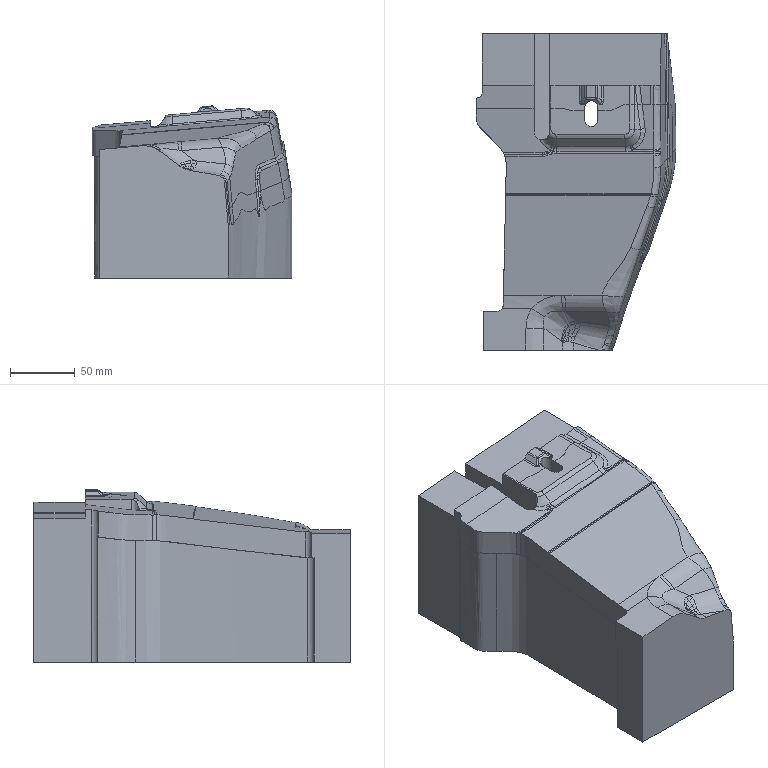Part | NX | features solid 2 | 1 solid | 199 faces | box 154.594 x 245 x 133.169 mm | volume 3383297 mm3 | spline 173 | plane 16 | cylinder 8 | sphere 2 | commonest cylinder face diameters 10 x5 12 x1 20 x1 25 x1